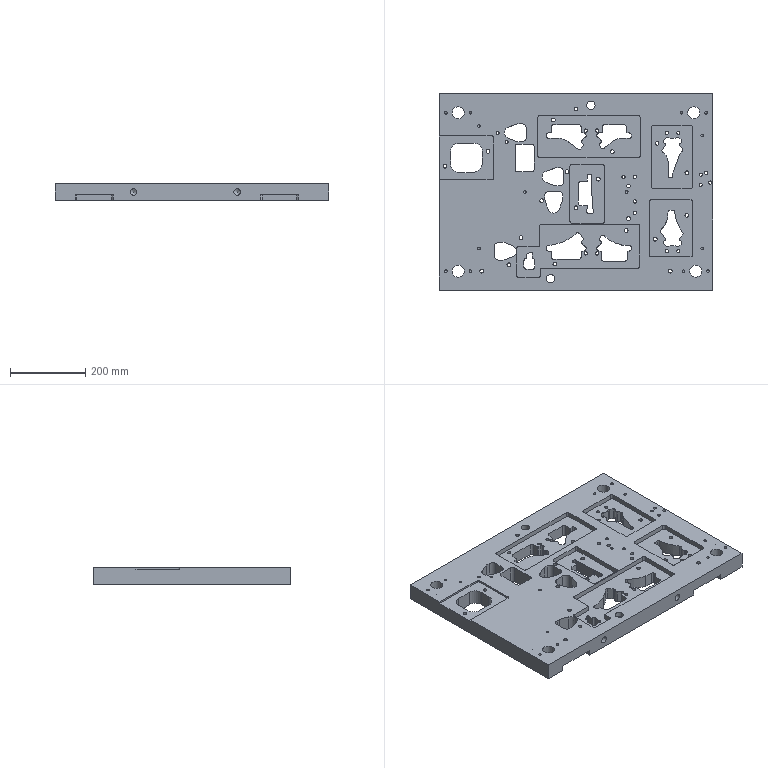Part | STEP file | 300_id70_x_t | 1 solid | 530 faces | box 725 x 520 x 45 mm | volume 13125415 mm3 | cylinder 273 | plane 164 | cone 69 | spline 24 | commonest cylinder face diameters 10 x65 8.5 x49 9 x36 6.8 x18 14 x18 1 x14